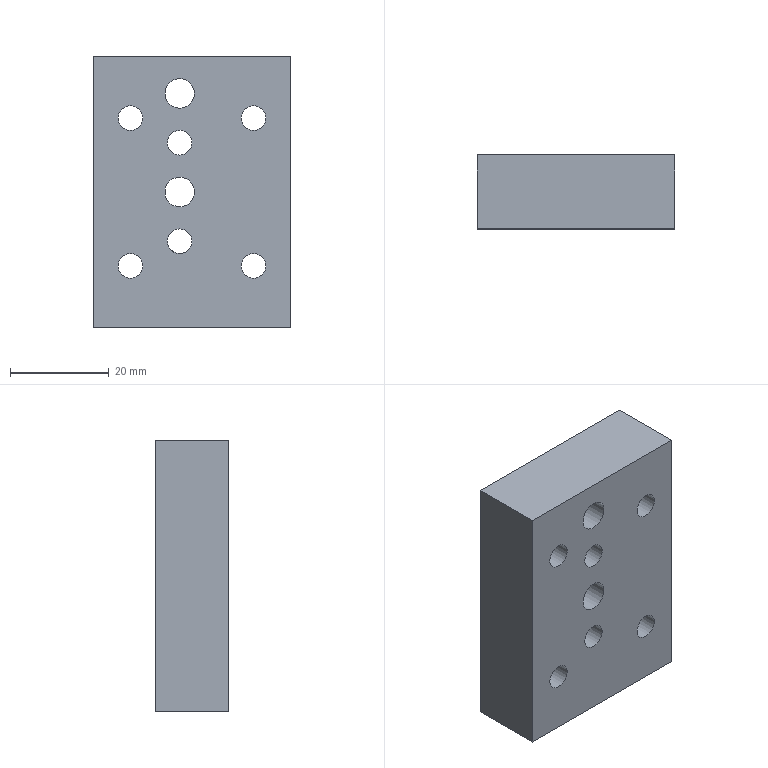Part | NX | features BREP 1 | 1 solid | 19 faces | box 40 x 15 x 55 mm | volume 29783 mm3 | cylinder 10 | plane 6 | cone 3 | commonest cylinder face diameters 5 x8 6 x2
STEP:
#1=CARTESIAN_POINT('',(-2.5,2.5,-12.5));
#2=VERTEX_POINT('',#1);
#3=CARTESIAN_POINT('',(-2.5,-2.5,-12.5));
#4=VERTEX_POINT('',#3);
#5=CARTESIAN_POINT('',(-2.5,0.,-12.5));
#6=DIRECTION('',(0.,0.,-1.));
#7=DIRECTION('',(-1.,0.,0.));
#8=AXIS2_PLACEMENT_3D('',#5,#6,#7);
#9=CIRCLE('',#8,2.5);
#10=EDGE_CURVE('',#2,#4,#9,.T.);
#11=ORIENTED_EDGE('',*,*,#10,.T.);
#12=CARTESIAN_POINT('',(-2.5,-2.5,-12.5));
#13=CARTESIAN_POINT('',(-2.221,-2.5,-12.5));
#14=CARTESIAN_POINT('',(-1.71,-2.239,-12.401));
#15=CARTESIAN_POINT('',(-1.104,-1.358,-12.105));
#16=CARTESIAN_POINT('',(-0.809,0.0009696,-11.835));
#17=CARTESIAN_POINT('',(-1.103,1.355,-12.105));
#18=CARTESIAN_POINT('',(-1.71,2.239,-12.401));
#19=CARTESIAN_POINT('',(-2.222,2.5,-12.5));
#20=CARTESIAN_POINT('',(-2.5,2.5,-12.5));
#21=B_SPLINE_CURVE_WITH_KNOTS('',3,(#12,#13,#14,#15,#16,#17,#18,#19,#20),.UNSPECIFIED.,.F.,.F.,(4,1,1,1,1,1,4),(0.,0.0008195,0.001639,0.003278,0.004917,0.005737,0.006556),.UNSPECIFIED.);
#22=EDGE_CURVE('',#4,#2,#21,.T.);
#23=ORIENTED_EDGE('',*,*,#22,.T.);
#24=EDGE_LOOP('',(#11,#23));
#25=FACE_BOUND('',#24,.T.);
#26=CARTESIAN_POINT('',(-2.5,0.,-12.5));
#27=DIRECTION('',(0.,0.,-1.));
#28=DIRECTION('',(1.,0.,0.));
#29=AXIS2_PLACEMENT_3D('',#26,#27,#28);
#30=CONICAL_SURFACE('',#29,2.5,1.03);
#31=ADVANCED_FACE('',(#25),#30,.F.);
#32=CARTESIAN_POINT('',(20.,0.,-2.5));
#33=VERTEX_POINT('',#32);
#34=CARTESIAN_POINT('',(20.,0.,0.));
#35=DIRECTION('',(1.,0.,0.));
#36=DIRECTION('',(0.,0.,-1.));
#37=AXIS2_PLACEMENT_3D('',#34,#35,#36);
#38=CIRCLE('',#37,2.5);
#39=EDGE_CURVE('',#33,#33,#38,.T.);
#40=ORIENTED_EDGE('',*,*,#39,.F.);
#41=EDGE_LOOP('',(#40));
#42=FACE_BOUND('',#41,.T.);
#43=CARTESIAN_POINT('',(20.,-7.5,27.5));
#44=VERTEX_POINT('',#43);
#45=CARTESIAN_POINT('',(20.,-7.5,-27.5));
#46=VERTEX_POINT('',#45);
#47=CARTESIAN_POINT('',(20.,-7.5,27.5));
#48=DIRECTION('',(0.,0.,-1.));
#49=VECTOR('',#48,1000.);
#50=LINE('',#47,#49);
#51=EDGE_CURVE('',#44,#46,#50,.T.);
#52=ORIENTED_EDGE('',*,*,#51,.T.);
#53=CARTESIAN_POINT('',(20.,7.5,-27.5));
#54=VERTEX_POINT('',#53);
#55=CARTESIAN_POINT('',(20.,7.5,-27.5));
#56=DIRECTION('',(0.,-1.,0.));
#57=VECTOR('',#56,1000.);
#58=LINE('',#55,#57);
#59=EDGE_CURVE('',#54,#46,#58,.T.);
#60=ORIENTED_EDGE('',*,*,#59,.F.);
#61=CARTESIAN_POINT('',(20.,7.5,27.5));
#62=VERTEX_POINT('',#61);
#63=CARTESIAN_POINT('',(20.,7.5,27.5));
#64=DIRECTION('',(0.,0.,-1.));
#65=VECTOR('',#64,1000.);
#66=LINE('',#63,#65);
#67=EDGE_CURVE('',#62,#54,#66,.T.);
#68=ORIENTED_EDGE('',*,*,#67,.F.);
#69=CARTESIAN_POINT('',(20.,7.5,27.5));
#70=DIRECTION('',(0.,-1.,0.));
#71=VECTOR('',#70,1000.);
#72=LINE('',#69,#71);
#73=EDGE_CURVE('',#62,#44,#72,.T.);
#74=ORIENTED_EDGE('',*,*,#73,.T.);
#75=EDGE_LOOP('',(#52,#60,#68,#74));
#76=FACE_BOUND('',#75,.T.);
#77=CARTESIAN_POINT('',(20.,7.5,27.5));
#78=DIRECTION('',(-1.,0.,0.));
#79=DIRECTION('',(0.,0.,-1.));
#80=AXIS2_PLACEMENT_3D('',#77,#78,#79);
#81=PLANE('',#80);
#82=ADVANCED_FACE('',(#42,#76),#81,.F.);
#83=CARTESIAN_POINT('',(-5.,0.,-27.5));
#84=VERTEX_POINT('',#83);
#85=CARTESIAN_POINT('',(-2.5,0.,-27.5));
#86=DIRECTION('',(0.,0.,-1.));
#87=DIRECTION('',(-1.,0.,0.));
#88=AXIS2_PLACEMENT_3D('',#85,#86,#87);
#89=CIRCLE('',#88,2.5);
#90=EDGE_CURVE('',#84,#84,#89,.T.);
#91=ORIENTED_EDGE('',*,*,#90,.F.);
#92=EDGE_LOOP('',(#91));
#93=FACE_BOUND('',#92,.T.);
#94=CARTESIAN_POINT('',(-20.,-7.5,-27.5));
#95=VERTEX_POINT('',#94);
#96=CARTESIAN_POINT('',(-20.,-7.5,-27.5));
#97=DIRECTION('',(-1.,0.,0.));
#98=VECTOR('',#97,1000.);
#99=LINE('',#96,#98);
#100=EDGE_CURVE('',#46,#95,#99,.T.);
#101=ORIENTED_EDGE('',*,*,#100,.T.);
#102=CARTESIAN_POINT('',(-20.,7.5,-27.5));
#103=VERTEX_POINT('',#102);
#104=CARTESIAN_POINT('',(-20.,7.5,-27.5));
#105=DIRECTION('',(0.,-1.,0.));
#106=VECTOR('',#105,1000.);
#107=LINE('',#104,#106);
#108=EDGE_CURVE('',#103,#95,#107,.T.);
#109=ORIENTED_EDGE('',*,*,#108,.F.);
#110=CARTESIAN_POINT('',(-20.,7.5,-27.5));
#111=DIRECTION('',(-1.,0.,0.));
#112=VECTOR('',#111,1000.);
#113=LINE('',#110,#112);
#114=EDGE_CURVE('',#54,#103,#113,.T.);
#115=ORIENTED_EDGE('',*,*,#114,.F.);
#116=ORIENTED_EDGE('',*,*,#59,.T.);
#117=EDGE_LOOP('',(#101,#109,#115,#116));
#118=FACE_BOUND('',#117,.T.);
#119=CARTESIAN_POINT('',(-20.,7.5,-27.5));
#120=DIRECTION('',(0.,0.,1.));
#121=DIRECTION('',(-1.,0.,0.));
#122=AXIS2_PLACEMENT_3D('',#119,#120,#121);
#123=PLANE('',#122);
#124=ADVANCED_FACE('',(#93,#118),#123,.F.);
#125=CARTESIAN_POINT('',(-20.,-7.5,27.5));
#126=VERTEX_POINT('',#125);
#127=CARTESIAN_POINT('',(-20.,-7.5,27.5));
#128=DIRECTION('',(0.,0.,1.));
#129=VECTOR('',#128,1000.);
#130=LINE('',#127,#129);
#131=EDGE_CURVE('',#95,#126,#130,.T.);
#132=ORIENTED_EDGE('',*,*,#131,.T.);
#133=CARTESIAN_POINT('',(-20.,7.5,27.5));
#134=VERTEX_POINT('',#133);
#135=CARTESIAN_POINT('',(-20.,7.5,27.5));
#136=DIRECTION('',(0.,-1.,0.));
#137=VECTOR('',#136,1000.);
#138=LINE('',#135,#137);
#139=EDGE_CURVE('',#134,#126,#138,.T.);
#140=ORIENTED_EDGE('',*,*,#139,.F.);
#141=CARTESIAN_POINT('',(-20.,7.5,27.5));
#142=DIRECTION('',(0.,0.,1.));
#143=VECTOR('',#142,1000.);
#144=LINE('',#141,#143);
#145=EDGE_CURVE('',#103,#134,#144,.T.);
#146=ORIENTED_EDGE('',*,*,#145,.F.);
#147=ORIENTED_EDGE('',*,*,#108,.T.);
#148=EDGE_LOOP('',(#132,#140,#146,#147));
#149=FACE_BOUND('',#148,.T.);
#150=CARTESIAN_POINT('',(-20.,7.5,27.5));
#151=DIRECTION('',(1.,0.,0.));
#152=DIRECTION('',(0.,0.,1.));
#153=AXIS2_PLACEMENT_3D('',#150,#151,#152);
#154=PLANE('',#153);
#155=ADVANCED_FACE('',(#149),#154,.F.);
#156=CARTESIAN_POINT('',(-20.,-7.5,27.5));
#157=DIRECTION('',(1.,0.,0.));
#158=VECTOR('',#157,1000.);
#159=LINE('',#156,#158);
#160=EDGE_CURVE('',#126,#44,#159,.T.);
#161=ORIENTED_EDGE('',*,*,#160,.T.);
#162=ORIENTED_EDGE('',*,*,#73,.F.);
#163=CARTESIAN_POINT('',(-20.,7.5,27.5));
#164=DIRECTION('',(1.,0.,0.));
#165=VECTOR('',#164,1000.);
#166=LINE('',#163,#165);
#167=EDGE_CURVE('',#134,#62,#166,.T.);
#168=ORIENTED_EDGE('',*,*,#167,.F.);
#169=ORIENTED_EDGE('',*,*,#139,.T.);
#170=EDGE_LOOP('',(#161,#162,#168,#169));
#171=FACE_BOUND('',#170,.T.);
#172=CARTESIAN_POINT('',(-20.,7.5,27.5));
#173=DIRECTION('',(0.,0.,-1.));
#174=DIRECTION('',(1.,0.,0.));
#175=AXIS2_PLACEMENT_3D('',#172,#173,#174);
#176=PLANE('',#175);
#177=ADVANCED_FACE('',(#171),#176,.F.);
#178=CARTESIAN_POINT('',(-12.5,7.5,-12.5));
#179=VERTEX_POINT('',#178);
#180=CARTESIAN_POINT('',(-12.5,7.5,-15.));
#181=DIRECTION('',(0.,1.,0.));
#182=DIRECTION('',(0.,0.,1.));
#183=AXIS2_PLACEMENT_3D('',#180,#181,#182);
#184=CIRCLE('',#183,2.5);
#185=EDGE_CURVE('',#179,#179,#184,.T.);
#186=ORIENTED_EDGE('',*,*,#185,.F.);
#187=EDGE_LOOP('',(#186));
#188=FACE_BOUND('',#187,.T.);
#189=CARTESIAN_POINT('',(12.5,7.5,17.5));
#190=VERTEX_POINT('',#189);
#191=CARTESIAN_POINT('',(12.5,7.5,15.));
#192=DIRECTION('',(0.,1.,0.));
#193=DIRECTION('',(0.,0.,1.));
#194=AXIS2_PLACEMENT_3D('',#191,#192,#193);
#195=CIRCLE('',#194,2.5);
#196=EDGE_CURVE('',#190,#190,#195,.T.);
#197=ORIENTED_EDGE('',*,*,#196,.F.);
#198=EDGE_LOOP('',(#197));
#199=FACE_BOUND('',#198,.T.);
#200=CARTESIAN_POINT('',(12.5,7.5,-12.5));
#201=VERTEX_POINT('',#200);
#202=CARTESIAN_POINT('',(12.5,7.5,-15.));
#203=DIRECTION('',(0.,1.,0.));
#204=DIRECTION('',(0.,0.,1.));
#205=AXIS2_PLACEMENT_3D('',#202,#203,#204);
#206=CIRCLE('',#205,2.5);
#207=EDGE_CURVE('',#201,#201,#206,.T.);
#208=ORIENTED_EDGE('',*,*,#207,.F.);
#209=EDGE_LOOP('',(#208));
#210=FACE_BOUND('',#209,.T.);
#211=CARTESIAN_POINT('',(-12.5,7.5,17.5));
#212=VERTEX_POINT('',#211);
#213=CARTESIAN_POINT('',(-12.5,7.5,15.));
#214=DIRECTION('',(0.,1.,0.));
#215=DIRECTION('',(0.,0.,1.));
#216=AXIS2_PLACEMENT_3D('',#213,#214,#215);
#217=CIRCLE('',#216,2.5);
#218=EDGE_CURVE('',#212,#212,#217,.T.);
#219=ORIENTED_EDGE('',*,*,#218,.F.);
#220=EDGE_LOOP('',(#219));
#221=FACE_BOUND('',#220,.T.);
#222=CARTESIAN_POINT('',(-2.5,7.5,12.5));
#223=VERTEX_POINT('',#222);
#224=CARTESIAN_POINT('',(-2.5,7.5,10.));
#225=DIRECTION('',(0.,1.,0.));
#226=DIRECTION('',(0.,0.,1.));
#227=AXIS2_PLACEMENT_3D('',#224,#225,#226);
#228=CIRCLE('',#227,2.5);
#229=EDGE_CURVE('',#223,#223,#228,.T.);
#230=ORIENTED_EDGE('',*,*,#229,.F.);
#231=EDGE_LOOP('',(#230));
#232=FACE_BOUND('',#231,.T.);
#233=CARTESIAN_POINT('',(-2.5,7.5,-7.5));
#234=VERTEX_POINT('',#233);
#235=CARTESIAN_POINT('',(-2.5,7.5,-10.));
#236=DIRECTION('',(0.,1.,0.));
#237=DIRECTION('',(0.,0.,1.));
#238=AXIS2_PLACEMENT_3D('',#235,#236,#237);
#239=CIRCLE('',#238,2.5);
#240=EDGE_CURVE('',#234,#234,#239,.T.);
#241=ORIENTED_EDGE('',*,*,#240,.F.);
#242=EDGE_LOOP('',(#241));
#243=FACE_BOUND('',#242,.T.);
#244=CARTESIAN_POINT('',(-2.5,7.5,3.));
#245=VERTEX_POINT('',#244);
#246=CARTESIAN_POINT('',(-2.5,7.5,0.));
#247=DIRECTION('',(0.,1.,0.));
#248=DIRECTION('',(0.,0.,1.));
#249=AXIS2_PLACEMENT_3D('',#246,#247,#248);
#250=CIRCLE('',#249,3.);
#251=EDGE_CURVE('',#245,#245,#250,.T.);
#252=ORIENTED_EDGE('',*,*,#251,.F.);
#253=EDGE_LOOP('',(#252));
#254=FACE_BOUND('',#253,.T.);
#255=CARTESIAN_POINT('',(-2.5,7.5,23.));
#256=VERTEX_POINT('',#255);
#257=CARTESIAN_POINT('',(-2.5,7.5,20.));
#258=DIRECTION('',(0.,1.,0.));
#259=DIRECTION('',(0.,0.,1.));
#260=AXIS2_PLACEMENT_3D('',#257,#258,#259);
#261=CIRCLE('',#260,3.);
#262=EDGE_CURVE('',#256,#256,#261,.T.);
#263=ORIENTED_EDGE('',*,*,#262,.F.);
#264=EDGE_LOOP('',(#263));
#265=FACE_BOUND('',#264,.T.);
#266=ORIENTED_EDGE('',*,*,#67,.T.);
#267=ORIENTED_EDGE('',*,*,#114,.T.);
#268=ORIENTED_EDGE('',*,*,#145,.T.);
#269=ORIENTED_EDGE('',*,*,#167,.T.);
#270=EDGE_LOOP('',(#266,#267,#268,#269));
#271=FACE_BOUND('',#270,.T.);
#272=CARTESIAN_POINT('',(0.,7.5,0.));
#273=DIRECTION('',(0.,-1.,0.));
#274=DIRECTION('',(0.,0.,1.));
#275=AXIS2_PLACEMENT_3D('',#272,#273,#274);
#276=PLANE('',#275);
#277=ADVANCED_FACE('',(#188,#199,#210,#221,#232,#243,#254,#265,#271),#276,.F.);
#278=CARTESIAN_POINT('',(-12.5,-7.5,-12.5));
#279=VERTEX_POINT('',#278);
#280=CARTESIAN_POINT('',(-12.5,-7.5,-15.));
#281=DIRECTION('',(0.,1.,0.));
#282=DIRECTION('',(0.,0.,1.));
#283=AXIS2_PLACEMENT_3D('',#280,#281,#282);
#284=CIRCLE('',#283,2.5);
#285=EDGE_CURVE('',#279,#279,#284,.T.);
#286=ORIENTED_EDGE('',*,*,#285,.T.);
#287=EDGE_LOOP('',(#286));
#288=FACE_BOUND('',#287,.T.);
#289=CARTESIAN_POINT('',(12.5,-7.5,17.5));
#290=VERTEX_POINT('',#289);
#291=CARTESIAN_POINT('',(12.5,-7.5,15.));
#292=DIRECTION('',(0.,1.,0.));
#293=DIRECTION('',(0.,0.,1.));
#294=AXIS2_PLACEMENT_3D('',#291,#292,#293);
#295=CIRCLE('',#294,2.5);
#296=EDGE_CURVE('',#290,#290,#295,.T.);
#297=ORIENTED_EDGE('',*,*,#296,.T.);
#298=EDGE_LOOP('',(#297));
#299=FACE_BOUND('',#298,.T.);
#300=CARTESIAN_POINT('',(12.5,-7.5,-12.5));
#301=VERTEX_POINT('',#300);
#302=CARTESIAN_POINT('',(12.5,-7.5,-15.));
#303=DIRECTION('',(0.,1.,0.));
#304=DIRECTION('',(0.,0.,1.));
#305=AXIS2_PLACEMENT_3D('',#302,#303,#304);
#306=CIRCLE('',#305,2.5);
#307=EDGE_CURVE('',#301,#301,#306,.T.);
#308=ORIENTED_EDGE('',*,*,#307,.T.);
#309=EDGE_LOOP('',(#308));
#310=FACE_BOUND('',#309,.T.);
#311=CARTESIAN_POINT('',(-12.5,-7.5,17.5));
#312=VERTEX_POINT('',#311);
#313=CARTESIAN_POINT('',(-12.5,-7.5,15.));
#314=DIRECTION('',(0.,1.,0.));
#315=DIRECTION('',(0.,0.,1.));
#316=AXIS2_PLACEMENT_3D('',#313,#314,#315);
#317=CIRCLE('',#316,2.5);
#318=EDGE_CURVE('',#312,#312,#317,.T.);
#319=ORIENTED_EDGE('',*,*,#318,.T.);
#320=EDGE_LOOP('',(#319));
#321=FACE_BOUND('',#320,.T.);
#322=CARTESIAN_POINT('',(-2.5,-7.5,12.5));
#323=VERTEX_POINT('',#322);
#324=CARTESIAN_POINT('',(-2.5,-7.5,10.));
#325=DIRECTION('',(0.,1.,0.));
#326=DIRECTION('',(0.,0.,1.));
#327=AXIS2_PLACEMENT_3D('',#324,#325,#326);
#328=CIRCLE('',#327,2.5);
#329=EDGE_CURVE('',#323,#323,#328,.T.);
#330=ORIENTED_EDGE('',*,*,#329,.T.);
#331=EDGE_LOOP('',(#330));
#332=FACE_BOUND('',#331,.T.);
#333=CARTESIAN_POINT('',(-2.5,-7.5,-7.5));
#334=VERTEX_POINT('',#333);
#335=CARTESIAN_POINT('',(-2.5,-7.5,-10.));
#336=DIRECTION('',(0.,1.,0.));
#337=DIRECTION('',(0.,0.,1.));
#338=AXIS2_PLACEMENT_3D('',#335,#336,#337);
#339=CIRCLE('',#338,2.5);
#340=EDGE_CURVE('',#334,#334,#339,.T.);
#341=ORIENTED_EDGE('',*,*,#340,.T.);
#342=EDGE_LOOP('',(#341));
#343=FACE_BOUND('',#342,.T.);
#344=CARTESIAN_POINT('',(-2.5,-7.5,3.));
#345=VERTEX_POINT('',#344);
#346=CARTESIAN_POINT('',(-2.5,-7.5,0.));
#347=DIRECTION('',(0.,1.,0.));
#348=DIRECTION('',(0.,0.,1.));
#349=AXIS2_PLACEMENT_3D('',#346,#347,#348);
#350=CIRCLE('',#349,3.);
#351=EDGE_CURVE('',#345,#345,#350,.T.);
#352=ORIENTED_EDGE('',*,*,#351,.T.);
#353=EDGE_LOOP('',(#352));
#354=FACE_BOUND('',#353,.T.);
#355=CARTESIAN_POINT('',(-2.5,-7.5,23.));
#356=VERTEX_POINT('',#355);
#357=CARTESIAN_POINT('',(-2.5,-7.5,20.));
#358=DIRECTION('',(0.,1.,0.));
#359=DIRECTION('',(0.,0.,1.));
#360=AXIS2_PLACEMENT_3D('',#357,#358,#359);
#361=CIRCLE('',#360,3.);
#362=EDGE_CURVE('',#356,#356,#361,.T.);
#363=ORIENTED_EDGE('',*,*,#362,.T.);
#364=EDGE_LOOP('',(#363));
#365=FACE_BOUND('',#364,.T.);
#366=ORIENTED_EDGE('',*,*,#51,.F.);
#367=ORIENTED_EDGE('',*,*,#160,.F.);
#368=ORIENTED_EDGE('',*,*,#131,.F.);
#369=ORIENTED_EDGE('',*,*,#100,.F.);
#370=EDGE_LOOP('',(#366,#367,#368,#369));
#371=FACE_BOUND('',#370,.T.);
#372=CARTESIAN_POINT('',(0.,-7.5,0.));
#373=DIRECTION('',(0.,-1.,0.));
#374=DIRECTION('',(0.,0.,1.));
#375=AXIS2_PLACEMENT_3D('',#372,#373,#374);
#376=PLANE('',#375);
#377=ADVANCED_FACE('',(#288,#299,#310,#321,#332,#343,#354,#365,#371),#376,.T.);
#378=CARTESIAN_POINT('',(3.498,0.,0.));
#379=VERTEX_POINT('',#378);
#380=VERTEX_LOOP('',#379);
#381=FACE_BOUND('',#380,.T.);
#382=CARTESIAN_POINT('',(5.,0.,-2.5));
#383=VERTEX_POINT('',#382);
#384=CARTESIAN_POINT('',(5.,0.,0.));
#385=DIRECTION('',(1.,0.,0.));
#386=DIRECTION('',(0.,0.,-1.));
#387=AXIS2_PLACEMENT_3D('',#384,#385,#386);
#388=CIRCLE('',#387,2.5);
#389=EDGE_CURVE('',#383,#383,#388,.T.);
#390=ORIENTED_EDGE('',*,*,#389,.T.);
#391=EDGE_LOOP('',(#390));
#392=FACE_BOUND('',#391,.T.);
#393=CARTESIAN_POINT('',(5.,0.,0.));
#394=DIRECTION('',(1.,0.,0.));
#395=DIRECTION('',(0.,0.,1.));
#396=AXIS2_PLACEMENT_3D('',#393,#394,#395);
#397=CONICAL_SURFACE('',#396,2.5,1.03);
#398=ADVANCED_FACE('',(#381,#392),#397,.F.);
#399=ORIENTED_EDGE('',*,*,#389,.F.);
#400=EDGE_LOOP('',(#399));
#401=FACE_BOUND('',#400,.T.);
#402=ORIENTED_EDGE('',*,*,#39,.T.);
#403=EDGE_LOOP('',(#402));
#404=FACE_BOUND('',#403,.T.);
#405=CARTESIAN_POINT('',(20.,0.,0.));
#406=DIRECTION('',(1.,0.,0.));
#407=DIRECTION('',(0.,0.,1.));
#408=AXIS2_PLACEMENT_3D('',#405,#406,#407);
#409=CYLINDRICAL_SURFACE('',#408,2.5);
#410=ADVANCED_FACE('',(#401,#404),#409,.F.);
#411=CARTESIAN_POINT('',(-2.5,0.,-12.5));
#412=DIRECTION('',(0.,0.,-1.));
#413=DIRECTION('',(-1.,0.,0.));
#414=AXIS2_PLACEMENT_3D('',#411,#412,#413);
#415=CIRCLE('',#414,2.5);
#416=EDGE_CURVE('',#4,#2,#415,.T.);
#417=ORIENTED_EDGE('',*,*,#416,.T.);
#418=CARTESIAN_POINT('',(-2.5,2.5,-12.5));
#419=CARTESIAN_POINT('',(-2.779,2.5,-12.5));
#420=CARTESIAN_POINT('',(-3.29,2.239,-12.401));
#421=CARTESIAN_POINT('',(-3.896,1.358,-12.105));
#422=CARTESIAN_POINT('',(-4.191,-0.0009696,-11.835));
#423=CARTESIAN_POINT('',(-3.897,-1.355,-12.105));
#424=CARTESIAN_POINT('',(-3.29,-2.239,-12.401));
#425=CARTESIAN_POINT('',(-2.778,-2.5,-12.5));
#426=CARTESIAN_POINT('',(-2.5,-2.5,-12.5));
#427=B_SPLINE_CURVE_WITH_KNOTS('',3,(#418,#419,#420,#421,#422,#423,#424,#425,#426),.UNSPECIFIED.,.F.,.F.,(4,1,1,1,1,1,4),(0.,0.0008195,0.001639,0.003278,0.004917,0.005737,0.006556),.UNSPECIFIED.);
#428=EDGE_CURVE('',#2,#4,#427,.T.);
#429=ORIENTED_EDGE('',*,*,#428,.T.);
#430=EDGE_LOOP('',(#417,#429));
#431=FACE_BOUND('',#430,.T.);
#432=CARTESIAN_POINT('',(-2.5,0.,-12.5));
#433=DIRECTION('',(0.,0.,-1.));
#434=DIRECTION('',(1.,0.,0.));
#435=AXIS2_PLACEMENT_3D('',#432,#433,#434);
#436=CONICAL_SURFACE('',#435,2.5,1.03);
#437=ADVANCED_FACE('',(#431),#436,.F.);
#438=ORIENTED_EDGE('',*,*,#10,.F.);
#439=ORIENTED_EDGE('',*,*,#416,.F.);
#440=EDGE_LOOP('',(#438,#439));
#441=FACE_BOUND('',#440,.T.);
#442=ORIENTED_EDGE('',*,*,#90,.T.);
#443=EDGE_LOOP('',(#442));
#444=FACE_BOUND('',#443,.T.);
#445=CARTESIAN_POINT('',(-2.5,0.,-27.5));
#446=DIRECTION('',(0.,0.,-1.));
#447=DIRECTION('',(1.,0.,0.));
#448=AXIS2_PLACEMENT_3D('',#445,#446,#447);
#449=CYLINDRICAL_SURFACE('',#448,2.5);
#450=ADVANCED_FACE('',(#441,#444),#449,.F.);
#451=ORIENTED_EDGE('',*,*,#362,.F.);
#452=EDGE_LOOP('',(#451));
#453=FACE_BOUND('',#452,.T.);
#454=ORIENTED_EDGE('',*,*,#262,.T.);
#455=EDGE_LOOP('',(#454));
#456=FACE_BOUND('',#455,.T.);
#457=CARTESIAN_POINT('',(-2.5,7.5,20.));
#458=DIRECTION('',(0.,1.,0.));
#459=DIRECTION('',(0.,0.,-1.));
#460=AXIS2_PLACEMENT_3D('',#457,#458,#459);
#461=CYLINDRICAL_SURFACE('',#460,3.);
#462=ADVANCED_FACE('',(#453,#456),#461,.F.);
#463=ORIENTED_EDGE('',*,*,#351,.F.);
#464=EDGE_LOOP('',(#463));
#465=FACE_BOUND('',#464,.T.);
#466=ORIENTED_EDGE('',*,*,#251,.T.);
#467=EDGE_LOOP('',(#466));
#468=FACE_BOUND('',#467,.T.);
#469=CARTESIAN_POINT('',(-2.5,7.5,0.));
#470=DIRECTION('',(0.,1.,0.));
#471=DIRECTION('',(0.,0.,-1.));
#472=AXIS2_PLACEMENT_3D('',#469,#470,#471);
#473=CYLINDRICAL_SURFACE('',#472,3.);
#474=ADVANCED_FACE('',(#465,#468),#473,.F.);
#475=ORIENTED_EDGE('',*,*,#340,.F.);
#476=EDGE_LOOP('',(#475));
#477=FACE_BOUND('',#476,.T.);
#478=ORIENTED_EDGE('',*,*,#240,.T.);
#479=EDGE_LOOP('',(#478));
#480=FACE_BOUND('',#479,.T.);
#481=ORIENTED_EDGE('',*,*,#428,.F.);
#482=ORIENTED_EDGE('',*,*,#22,.F.);
#483=EDGE_LOOP('',(#481,#482));
#484=FACE_BOUND('',#483,.T.);
#485=CARTESIAN_POINT('',(-2.5,7.5,-10.));
#486=DIRECTION('',(0.,1.,0.));
#487=DIRECTION('',(0.,0.,-1.));
#488=AXIS2_PLACEMENT_3D('',#485,#486,#487);
#489=CYLINDRICAL_SURFACE('',#488,2.5);
#490=ADVANCED_FACE('',(#477,#480,#484),#489,.F.);
#491=ORIENTED_EDGE('',*,*,#329,.F.);
#492=EDGE_LOOP('',(#491));
#493=FACE_BOUND('',#492,.T.);
#494=ORIENTED_EDGE('',*,*,#229,.T.);
#495=EDGE_LOOP('',(#494));
#496=FACE_BOUND('',#495,.T.);
#497=CARTESIAN_POINT('',(-2.5,7.5,10.));
#498=DIRECTION('',(0.,1.,0.));
#499=DIRECTION('',(0.,0.,-1.));
#500=AXIS2_PLACEMENT_3D('',#497,#498,#499);
#501=CYLINDRICAL_SURFACE('',#500,2.5);
#502=ADVANCED_FACE('',(#493,#496),#501,.F.);
#503=ORIENTED_EDGE('',*,*,#318,.F.);
#504=EDGE_LOOP('',(#503));
#505=FACE_BOUND('',#504,.T.);
#506=ORIENTED_EDGE('',*,*,#218,.T.);
#507=EDGE_LOOP('',(#506));
#508=FACE_BOUND('',#507,.T.);
#509=CARTESIAN_POINT('',(-12.5,7.5,15.));
#510=DIRECTION('',(0.,1.,0.));
#511=DIRECTION('',(0.,0.,-1.));
#512=AXIS2_PLACEMENT_3D('',#509,#510,#511);
#513=CYLINDRICAL_SURFACE('',#512,2.5);
#514=ADVANCED_FACE('',(#505,#508),#513,.F.);
#515=ORIENTED_EDGE('',*,*,#307,.F.);
#516=EDGE_LOOP('',(#515));
#517=FACE_BOUND('',#516,.T.);
#518=ORIENTED_EDGE('',*,*,#207,.T.);
#519=EDGE_LOOP('',(#518));
#520=FACE_BOUND('',#519,.T.);
#521=CARTESIAN_POINT('',(12.5,7.5,-15.));
#522=DIRECTION('',(0.,1.,0.));
#523=DIRECTION('',(0.,0.,-1.));
#524=AXIS2_PLACEMENT_3D('',#521,#522,#523);
#525=CYLINDRICAL_SURFACE('',#524,2.5);
#526=ADVANCED_FACE('',(#517,#520),#525,.F.);
#527=ORIENTED_EDGE('',*,*,#296,.F.);
#528=EDGE_LOOP('',(#527));
#529=FACE_BOUND('',#528,.T.);
#530=ORIENTED_EDGE('',*,*,#196,.T.);
#531=EDGE_LOOP('',(#530));
#532=FACE_BOUND('',#531,.T.);
#533=CARTESIAN_POINT('',(12.5,7.5,15.));
#534=DIRECTION('',(0.,1.,0.));
#535=DIRECTION('',(0.,0.,-1.));
#536=AXIS2_PLACEMENT_3D('',#533,#534,#535);
#537=CYLINDRICAL_SURFACE('',#536,2.5);
#538=ADVANCED_FACE('',(#529,#532),#537,.F.);
#539=ORIENTED_EDGE('',*,*,#285,.F.);
#540=EDGE_LOOP('',(#539));
#541=FACE_BOUND('',#540,.T.);
#542=ORIENTED_EDGE('',*,*,#185,.T.);
#543=EDGE_LOOP('',(#542));
#544=FACE_BOUND('',#543,.T.);
#545=CARTESIAN_POINT('',(-12.5,7.5,-15.));
#546=DIRECTION('',(0.,1.,0.));
#547=DIRECTION('',(0.,0.,-1.));
#548=AXIS2_PLACEMENT_3D('',#545,#546,#547);
#549=CYLINDRICAL_SURFACE('',#548,2.5);
#550=ADVANCED_FACE('',(#541,#544),#549,.F.);
#551=CLOSED_SHELL('',(#31,#82,#124,#155,#177,#277,#377,#398,#410,#437,#450,#462,#474,#490,#502,#514,#526,#538,#550));
#552=MANIFOLD_SOLID_BREP('',#551);
#553=(LENGTH_UNIT()NAMED_UNIT(*)SI_UNIT(.MILLI.,.METRE.));
#554=UNCERTAINTY_MEASURE_WITH_UNIT(LENGTH_MEASURE(0.0508),#553,'','');
#555=(NAMED_UNIT(*)PLANE_ANGLE_UNIT()SI_UNIT($,.RADIAN.));
#556=(NAMED_UNIT(*)SI_UNIT($,.STERADIAN.)SOLID_ANGLE_UNIT());
#557=(GEOMETRIC_REPRESENTATION_CONTEXT(3)GLOBAL_UNCERTAINTY_ASSIGNED_CONTEXT((#554))GLOBAL_UNIT_ASSIGNED_CONTEXT((#553,#555,#556))REPRESENTATION_CONTEXT('',''));
#558=ADVANCED_BREP_SHAPE_REPRESENTATION('',(#552),#557);